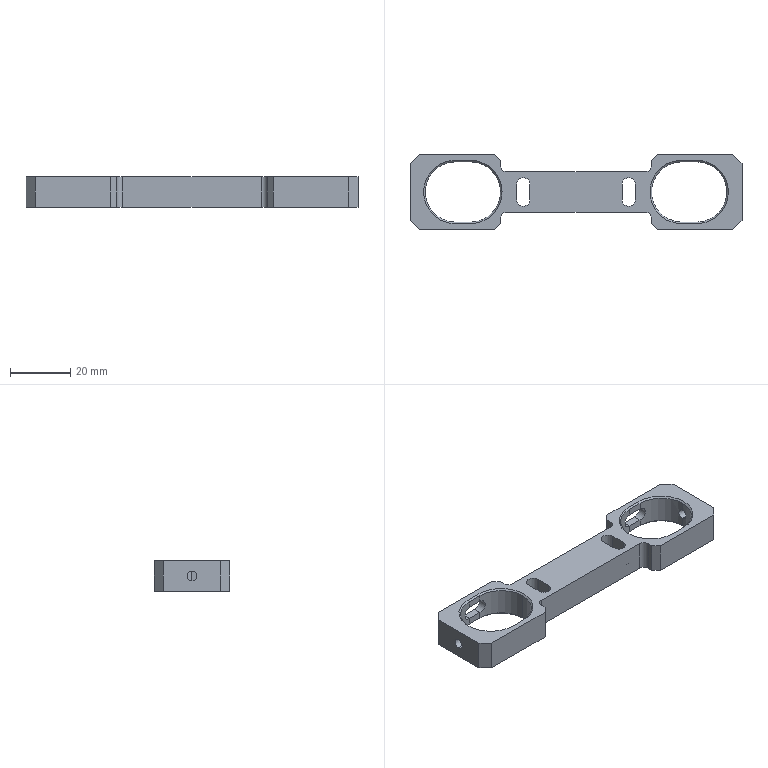Part | SolidWorks | features ICE 5, Chamfer 3, HoleWzd 2, Extrusion 1, Fillet 1 | 1 solid | 88 faces | box 110 x 25 x 10 mm | volume 11689 mm3 | plane 50 | cylinder 26 | cone 12 | commonest cylinder face diameters 4.5 x8 20 x6 3.3 x4 4 x4 8 x4